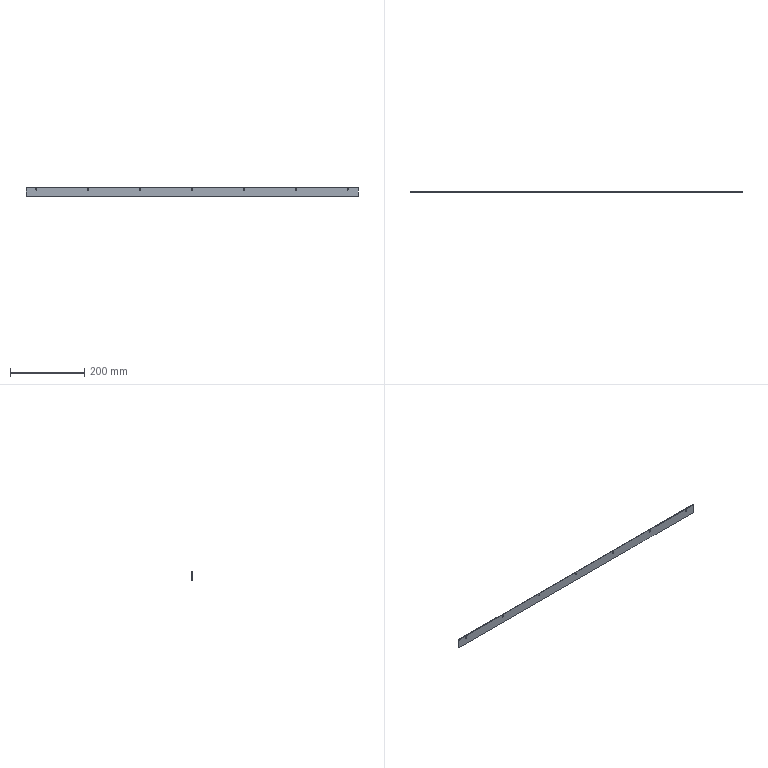Part | STEP file | BZJ-BZMM-JDKTBDYY Product限位Plate二 | 1 solid | 38 faces | box 895 x 2 x 26 mm | volume 46280 mm3 | cylinder 18 | cone 14 | plane 6 | commonest cylinder face diameters 3.4 x14 4 x4